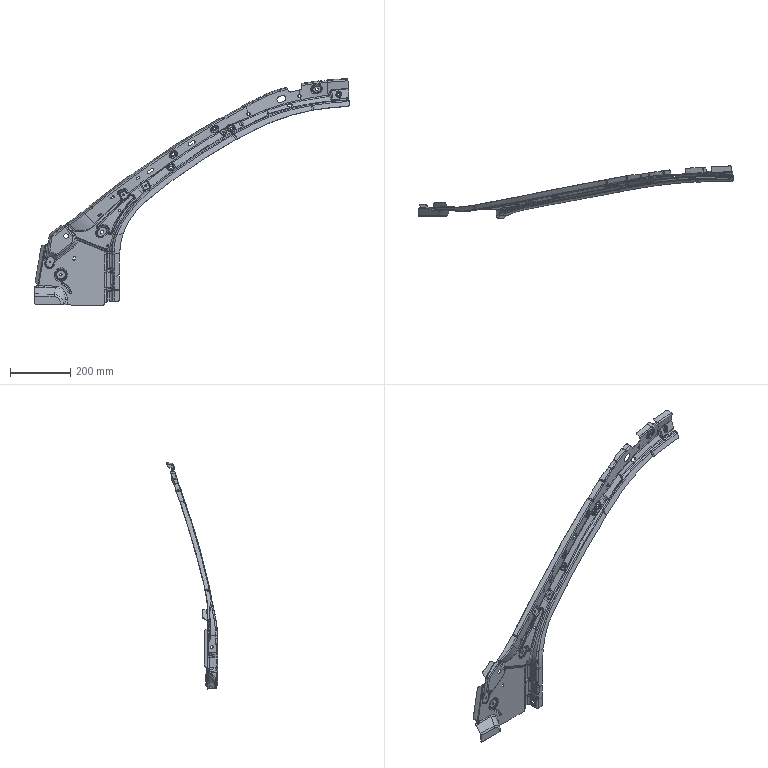Part | STEP file | FNA5401351 | 1 solid | 1337 faces | box 1045 x 172.359 x 753.685 mm | volume 232138 mm3 | spline 1055 | cylinder 176 | plane 70 | sphere 22 | other 10 | torus 4 | commonest cylinder face diameters 7 x16 6 x14 12 x14 8.4 x11 18 x11 8 x10